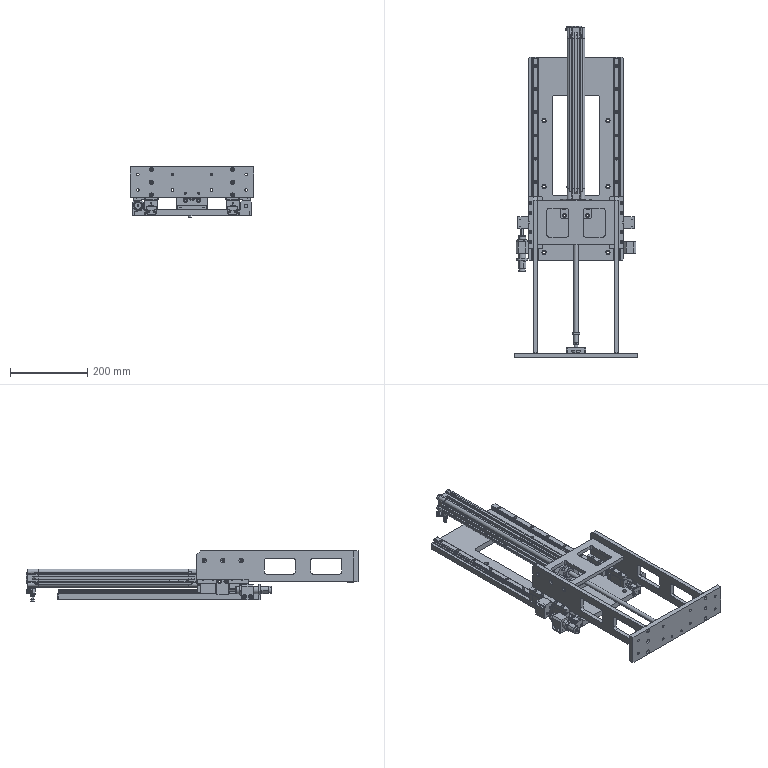Part | SolidWorks | 30 solids | 1983 faces | box 320 x 857.77 x 130.25 mm | volume 3607069 mm3 | cylinder 866 | plane 830 | cone 276 | spline 11 | commonest cylinder face diameters 1 x92 3.3 x92 4.5 x76 11 x66 6.6 x60 10 x54